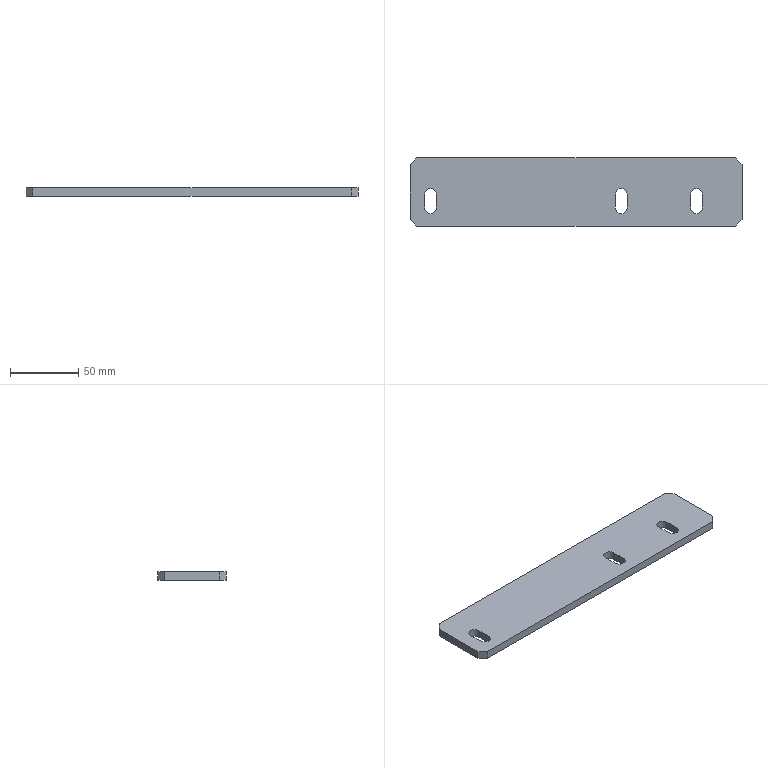Part | STEP file | 1_id978_x_t | 1 solid | 22 faces | box 243 x 50 x 6 mm | volume 70049 mm3 | plane 16 | cylinder 6 | commonest cylinder face diameters 8.5 x6